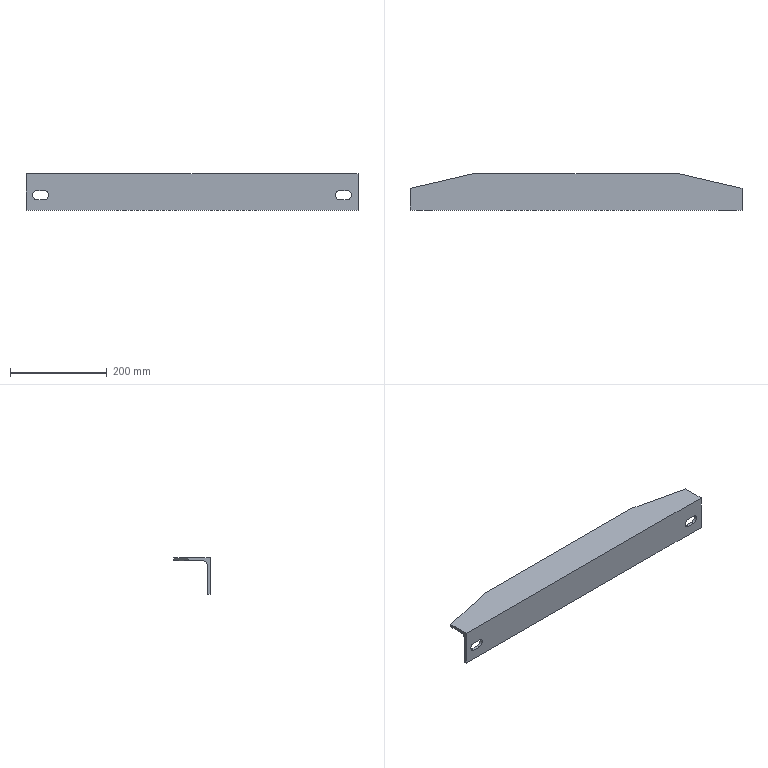Part | SolidWorks | features Chamfer 2, ICE 2, WeldMemberFeat 1, WeldmentFeature 1 | 1 solid | 21 faces | box 686 x 75 x 75 mm | volume 573977 mm3 | plane 14 | cylinder 7 | commonest cylinder face diameters 18 x5 4 x2
STEP:
#1=CARTESIAN_POINT('',(213.,75.,-4.));
#2=VERTEX_POINT('',#1);
#3=CARTESIAN_POINT('',(-213.,75.,-4.));
#4=VERTEX_POINT('',#3);
#5=CARTESIAN_POINT('',(343.,75.,-4.));
#6=DIRECTION('',(-1.,0.,0.));
#7=VECTOR('',#6,1000.);
#8=LINE('',#5,#7);
#9=EDGE_CURVE('',#2,#4,#8,.T.);
#10=ORIENTED_EDGE('',*,*,#9,.T.);
#11=CARTESIAN_POINT('',(-213.,75.,0.));
#12=VERTEX_POINT('',#11);
#13=CARTESIAN_POINT('',(-213.,75.,0.));
#14=DIRECTION('',(0.,0.,1.));
#15=VECTOR('',#14,1000.);
#16=LINE('',#13,#15);
#17=EDGE_CURVE('',#4,#12,#16,.T.);
#18=ORIENTED_EDGE('',*,*,#17,.T.);
#19=CARTESIAN_POINT('',(213.,75.,0.));
#20=VERTEX_POINT('',#19);
#21=CARTESIAN_POINT('',(343.,75.,0.));
#22=DIRECTION('',(-1.,0.,0.));
#23=VECTOR('',#22,1000.);
#24=LINE('',#21,#23);
#25=EDGE_CURVE('',#20,#12,#24,.T.);
#26=ORIENTED_EDGE('',*,*,#25,.F.);
#27=CARTESIAN_POINT('',(213.,75.,0.));
#28=DIRECTION('',(0.,0.,-1.));
#29=VECTOR('',#28,1000.);
#30=LINE('',#27,#29);
#31=EDGE_CURVE('',#20,#2,#30,.T.);
#32=ORIENTED_EDGE('',*,*,#31,.T.);
#33=EDGE_LOOP('',(#10,#18,#26,#32));
#34=FACE_OUTER_BOUND('',#33,.T.);
#35=CARTESIAN_POINT('',(343.,75.,0.));
#36=DIRECTION('',(0.,-1.,0.));
#37=DIRECTION('',(0.,0.,-1.));
#38=AXIS2_PLACEMENT_3D('',#35,#36,#37);
#39=PLANE('',#38);
#40=ADVANCED_FACE('',(#34),#39,.F.);
#41=ORIENTED_EDGE('',*,*,#25,.T.);
#42=CARTESIAN_POINT('',(-343.,45.,0.));
#43=VERTEX_POINT('',#42);
#44=CARTESIAN_POINT('',(-213.,75.,0.));
#45=DIRECTION('',(-0.9744,-0.2249,0.));
#46=VECTOR('',#45,1000.);
#47=LINE('',#44,#46);
#48=EDGE_CURVE('',#12,#43,#47,.T.);
#49=ORIENTED_EDGE('',*,*,#48,.T.);
#50=CARTESIAN_POINT('',(-343.,0.,0.));
#51=VERTEX_POINT('',#50);
#52=CARTESIAN_POINT('',(-343.,75.,0.));
#53=DIRECTION('',(0.,-1.,0.));
#54=VECTOR('',#53,1000.);
#55=LINE('',#52,#54);
#56=EDGE_CURVE('',#43,#51,#55,.T.);
#57=ORIENTED_EDGE('',*,*,#56,.T.);
#58=CARTESIAN_POINT('',(343.,0.,0.));
#59=VERTEX_POINT('',#58);
#60=CARTESIAN_POINT('',(343.,0.,0.));
#61=DIRECTION('',(-1.,0.,0.));
#62=VECTOR('',#61,1000.);
#63=LINE('',#60,#62);
#64=EDGE_CURVE('',#59,#51,#63,.T.);
#65=ORIENTED_EDGE('',*,*,#64,.F.);
#66=CARTESIAN_POINT('',(343.,45.,0.));
#67=VERTEX_POINT('',#66);
#68=CARTESIAN_POINT('',(343.,75.,0.));
#69=DIRECTION('',(0.,-1.,0.));
#70=VECTOR('',#69,1000.);
#71=LINE('',#68,#70);
#72=EDGE_CURVE('',#67,#59,#71,.T.);
#73=ORIENTED_EDGE('',*,*,#72,.F.);
#74=CARTESIAN_POINT('',(343.,45.,0.));
#75=DIRECTION('',(-0.9744,0.2249,0.));
#76=VECTOR('',#75,1000.);
#77=LINE('',#74,#76);
#78=EDGE_CURVE('',#67,#20,#77,.T.);
#79=ORIENTED_EDGE('',*,*,#78,.T.);
#80=EDGE_LOOP('',(#41,#49,#57,#65,#73,#79));
#81=FACE_OUTER_BOUND('',#80,.T.);
#82=CARTESIAN_POINT('',(343.,75.,0.));
#83=DIRECTION('',(0.,0.,-1.));
#84=DIRECTION('',(0.,1.,0.));
#85=AXIS2_PLACEMENT_3D('',#82,#83,#84);
#86=PLANE('',#85);
#87=ADVANCED_FACE('',(#81),#86,.F.);
#88=CARTESIAN_POINT('',(-320.5,0.,-53.));
#89=VERTEX_POINT('',#88);
#90=CARTESIAN_POINT('',(-305.5,0.,-53.));
#91=VERTEX_POINT('',#90);
#92=CARTESIAN_POINT('',(-320.5,0.,-53.));
#93=DIRECTION('',(1.,0.,0.));
#94=VECTOR('',#93,1000.);
#95=LINE('',#92,#94);
#96=EDGE_CURVE('',#89,#91,#95,.T.);
#97=ORIENTED_EDGE('',*,*,#96,.F.);
#98=CARTESIAN_POINT('',(-320.5,0.,-35.));
#99=VERTEX_POINT('',#98);
#100=CARTESIAN_POINT('',(-320.5,0.,-44.));
#101=DIRECTION('',(0.,-1.,0.));
#102=DIRECTION('',(0.,0.,1.));
#103=AXIS2_PLACEMENT_3D('',#100,#101,#102);
#104=CIRCLE('',#103,9.);
#105=EDGE_CURVE('',#99,#89,#104,.T.);
#106=ORIENTED_EDGE('',*,*,#105,.F.);
#107=CARTESIAN_POINT('',(-305.5,0.,-35.));
#108=VERTEX_POINT('',#107);
#109=CARTESIAN_POINT('',(-320.5,0.,-35.));
#110=DIRECTION('',(-1.,0.,0.));
#111=VECTOR('',#110,1000.);
#112=LINE('',#109,#111);
#113=EDGE_CURVE('',#108,#99,#112,.T.);
#114=ORIENTED_EDGE('',*,*,#113,.F.);
#115=CARTESIAN_POINT('',(-305.5,0.,-44.));
#116=DIRECTION('',(0.,-1.,0.));
#117=DIRECTION('',(0.,0.,1.));
#118=AXIS2_PLACEMENT_3D('',#115,#116,#117);
#119=CIRCLE('',#118,9.);
#120=EDGE_CURVE('',#91,#108,#119,.T.);
#121=ORIENTED_EDGE('',*,*,#120,.F.);
#122=EDGE_LOOP('',(#97,#106,#114,#121));
#123=FACE_BOUND('',#122,.T.);
#124=CARTESIAN_POINT('',(305.5,0.,-53.));
#125=VERTEX_POINT('',#124);
#126=CARTESIAN_POINT('',(320.5,0.,-53.));
#127=VERTEX_POINT('',#126);
#128=CARTESIAN_POINT('',(305.5,0.,-53.));
#129=DIRECTION('',(1.,0.,0.));
#130=VECTOR('',#129,1000.);
#131=LINE('',#128,#130);
#132=EDGE_CURVE('',#125,#127,#131,.T.);
#133=ORIENTED_EDGE('',*,*,#132,.F.);
#134=CARTESIAN_POINT('',(305.5,0.,-35.));
#135=VERTEX_POINT('',#134);
#136=CARTESIAN_POINT('',(305.5,0.,-44.));
#137=DIRECTION('',(0.,-1.,0.));
#138=DIRECTION('',(0.,0.,1.));
#139=AXIS2_PLACEMENT_3D('',#136,#137,#138);
#140=CIRCLE('',#139,9.);
#141=EDGE_CURVE('',#135,#125,#140,.T.);
#142=ORIENTED_EDGE('',*,*,#141,.F.);
#143=CARTESIAN_POINT('',(320.5,0.,-35.));
#144=VERTEX_POINT('',#143);
#145=CARTESIAN_POINT('',(305.5,0.,-35.));
#146=DIRECTION('',(-1.,0.,0.));
#147=VECTOR('',#146,1000.);
#148=LINE('',#145,#147);
#149=EDGE_CURVE('',#144,#135,#148,.T.);
#150=ORIENTED_EDGE('',*,*,#149,.F.);
#151=CARTESIAN_POINT('',(320.5,0.,-44.));
#152=DIRECTION('',(0.,-1.,0.));
#153=DIRECTION('',(0.,0.,1.));
#154=AXIS2_PLACEMENT_3D('',#151,#152,#153);
#155=CIRCLE('',#154,9.);
#156=EDGE_CURVE('',#127,#144,#155,.T.);
#157=ORIENTED_EDGE('',*,*,#156,.F.);
#158=EDGE_LOOP('',(#133,#142,#150,#157));
#159=FACE_BOUND('',#158,.T.);
#160=CARTESIAN_POINT('',(-343.,0.,-75.));
#161=VERTEX_POINT('',#160);
#162=CARTESIAN_POINT('',(-343.,0.,0.));
#163=DIRECTION('',(0.,0.,-1.));
#164=VECTOR('',#163,1000.);
#165=LINE('',#162,#164);
#166=EDGE_CURVE('',#51,#161,#165,.T.);
#167=ORIENTED_EDGE('',*,*,#166,.T.);
#168=CARTESIAN_POINT('',(343.,0.,-75.));
#169=VERTEX_POINT('',#168);
#170=CARTESIAN_POINT('',(343.,0.,-75.));
#171=DIRECTION('',(-1.,0.,0.));
#172=VECTOR('',#171,1000.);
#173=LINE('',#170,#172);
#174=EDGE_CURVE('',#169,#161,#173,.T.);
#175=ORIENTED_EDGE('',*,*,#174,.F.);
#176=CARTESIAN_POINT('',(343.,0.,0.));
#177=DIRECTION('',(0.,0.,-1.));
#178=VECTOR('',#177,1000.);
#179=LINE('',#176,#178);
#180=EDGE_CURVE('',#59,#169,#179,.T.);
#181=ORIENTED_EDGE('',*,*,#180,.F.);
#182=ORIENTED_EDGE('',*,*,#64,.T.);
#183=EDGE_LOOP('',(#167,#175,#181,#182));
#184=FACE_OUTER_BOUND('',#183,.T.);
#185=CARTESIAN_POINT('',(343.,0.,0.));
#186=DIRECTION('',(0.,1.,0.));
#187=DIRECTION('',(0.,0.,1.));
#188=AXIS2_PLACEMENT_3D('',#185,#186,#187);
#189=PLANE('',#188);
#190=ADVANCED_FACE('',(#123,#159,#184),#189,.F.);
#191=CARTESIAN_POINT('',(-343.,4.,-75.));
#192=VERTEX_POINT('',#191);
#193=CARTESIAN_POINT('',(-343.,0.,-75.));
#194=DIRECTION('',(0.,1.,0.));
#195=VECTOR('',#194,1000.);
#196=LINE('',#193,#195);
#197=EDGE_CURVE('',#161,#192,#196,.T.);
#198=ORIENTED_EDGE('',*,*,#197,.T.);
#199=CARTESIAN_POINT('',(343.,4.,-75.));
#200=VERTEX_POINT('',#199);
#201=CARTESIAN_POINT('',(343.,4.,-75.));
#202=DIRECTION('',(-1.,0.,0.));
#203=VECTOR('',#202,1000.);
#204=LINE('',#201,#203);
#205=EDGE_CURVE('',#200,#192,#204,.T.);
#206=ORIENTED_EDGE('',*,*,#205,.F.);
#207=CARTESIAN_POINT('',(343.,0.,-75.));
#208=DIRECTION('',(0.,1.,0.));
#209=VECTOR('',#208,1000.);
#210=LINE('',#207,#209);
#211=EDGE_CURVE('',#169,#200,#210,.T.);
#212=ORIENTED_EDGE('',*,*,#211,.F.);
#213=ORIENTED_EDGE('',*,*,#174,.T.);
#214=EDGE_LOOP('',(#198,#206,#212,#213));
#215=FACE_OUTER_BOUND('',#214,.T.);
#216=CARTESIAN_POINT('',(343.,0.,-75.));
#217=DIRECTION('',(0.,0.,1.));
#218=DIRECTION('',(0.,-1.,0.));
#219=AXIS2_PLACEMENT_3D('',#216,#217,#218);
#220=PLANE('',#219);
#221=ADVANCED_FACE('',(#215),#220,.F.);
#222=CARTESIAN_POINT('',(-343.,6.,-73.));
#223=VERTEX_POINT('',#222);
#224=CARTESIAN_POINT('',(-343.,4.,-73.));
#225=DIRECTION('',(1.,0.,0.));
#226=DIRECTION('',(0.,0.,-1.));
#227=AXIS2_PLACEMENT_3D('',#224,#225,#226);
#228=CIRCLE('',#227,2.);
#229=EDGE_CURVE('',#192,#223,#228,.T.);
#230=ORIENTED_EDGE('',*,*,#229,.T.);
#231=CARTESIAN_POINT('',(343.,6.,-73.));
#232=VERTEX_POINT('',#231);
#233=CARTESIAN_POINT('',(343.,6.,-73.));
#234=DIRECTION('',(-1.,0.,0.));
#235=VECTOR('',#234,1000.);
#236=LINE('',#233,#235);
#237=EDGE_CURVE('',#232,#223,#236,.T.);
#238=ORIENTED_EDGE('',*,*,#237,.F.);
#239=CARTESIAN_POINT('',(343.,4.,-73.));
#240=DIRECTION('',(1.,0.,0.));
#241=DIRECTION('',(0.,0.,-1.));
#242=AXIS2_PLACEMENT_3D('',#239,#240,#241);
#243=CIRCLE('',#242,2.);
#244=EDGE_CURVE('',#200,#232,#243,.T.);
#245=ORIENTED_EDGE('',*,*,#244,.F.);
#246=ORIENTED_EDGE('',*,*,#205,.T.);
#247=EDGE_LOOP('',(#230,#238,#245,#246));
#248=FACE_OUTER_BOUND('',#247,.T.);
#249=CARTESIAN_POINT('',(343.,4.,-73.));
#250=DIRECTION('',(-1.,0.,0.));
#251=DIRECTION('',(0.,0.,1.));
#252=AXIS2_PLACEMENT_3D('',#249,#250,#251);
#253=CYLINDRICAL_SURFACE('',#252,2.);
#254=ADVANCED_FACE('',(#248),#253,.T.);
#255=CARTESIAN_POINT('',(-320.5,6.,-35.));
#256=VERTEX_POINT('',#255);
#257=CARTESIAN_POINT('',(-305.5,6.,-35.));
#258=VERTEX_POINT('',#257);
#259=CARTESIAN_POINT('',(-320.5,6.,-35.));
#260=DIRECTION('',(1.,0.,0.));
#261=VECTOR('',#260,1000.);
#262=LINE('',#259,#261);
#263=EDGE_CURVE('',#256,#258,#262,.T.);
#264=ORIENTED_EDGE('',*,*,#263,.F.);
#265=CARTESIAN_POINT('',(-320.5,6.,-53.));
#266=VERTEX_POINT('',#265);
#267=CARTESIAN_POINT('',(-320.5,6.,-44.));
#268=DIRECTION('',(0.,1.,0.));
#269=DIRECTION('',(0.,0.,1.));
#270=AXIS2_PLACEMENT_3D('',#267,#268,#269);
#271=CIRCLE('',#270,9.);
#272=EDGE_CURVE('',#266,#256,#271,.T.);
#273=ORIENTED_EDGE('',*,*,#272,.F.);
#274=CARTESIAN_POINT('',(-305.5,6.,-53.));
#275=VERTEX_POINT('',#274);
#276=CARTESIAN_POINT('',(-320.5,6.,-53.));
#277=DIRECTION('',(-1.,0.,0.));
#278=VECTOR('',#277,1000.);
#279=LINE('',#276,#278);
#280=EDGE_CURVE('',#275,#266,#279,.T.);
#281=ORIENTED_EDGE('',*,*,#280,.F.);
#282=CARTESIAN_POINT('',(-305.5,6.,-44.));
#283=DIRECTION('',(0.,1.,0.));
#284=DIRECTION('',(0.,0.,1.));
#285=AXIS2_PLACEMENT_3D('',#282,#283,#284);
#286=CIRCLE('',#285,9.);
#287=EDGE_CURVE('',#258,#275,#286,.T.);
#288=ORIENTED_EDGE('',*,*,#287,.F.);
#289=EDGE_LOOP('',(#264,#273,#281,#288));
#290=FACE_BOUND('',#289,.T.);
#291=CARTESIAN_POINT('',(305.5,6.,-35.));
#292=VERTEX_POINT('',#291);
#293=CARTESIAN_POINT('',(320.5,6.,-35.));
#294=VERTEX_POINT('',#293);
#295=CARTESIAN_POINT('',(305.5,6.,-35.));
#296=DIRECTION('',(1.,0.,0.));
#297=VECTOR('',#296,1000.);
#298=LINE('',#295,#297);
#299=EDGE_CURVE('',#292,#294,#298,.T.);
#300=ORIENTED_EDGE('',*,*,#299,.F.);
#301=CARTESIAN_POINT('',(305.5,6.,-53.));
#302=VERTEX_POINT('',#301);
#303=CARTESIAN_POINT('',(305.5,6.,-44.));
#304=DIRECTION('',(0.,1.,0.));
#305=DIRECTION('',(0.,0.,1.));
#306=AXIS2_PLACEMENT_3D('',#303,#304,#305);
#307=CIRCLE('',#306,9.);
#308=EDGE_CURVE('',#302,#292,#307,.T.);
#309=ORIENTED_EDGE('',*,*,#308,.F.);
#310=CARTESIAN_POINT('',(320.5,6.,-53.));
#311=VERTEX_POINT('',#310);
#312=CARTESIAN_POINT('',(305.5,6.,-53.));
#313=DIRECTION('',(-1.,0.,0.));
#314=VECTOR('',#313,1000.);
#315=LINE('',#312,#314);
#316=EDGE_CURVE('',#311,#302,#315,.T.);
#317=ORIENTED_EDGE('',*,*,#316,.F.);
#318=CARTESIAN_POINT('',(320.5,6.,-44.));
#319=DIRECTION('',(0.,1.,0.));
#320=DIRECTION('',(0.,0.,1.));
#321=AXIS2_PLACEMENT_3D('',#318,#319,#320);
#322=CIRCLE('',#321,9.);
#323=EDGE_CURVE('',#294,#311,#322,.T.);
#324=ORIENTED_EDGE('',*,*,#323,.F.);
#325=EDGE_LOOP('',(#300,#309,#317,#324));
#326=FACE_BOUND('',#325,.T.);
#327=CARTESIAN_POINT('',(-343.,6.,-15.));
#328=VERTEX_POINT('',#327);
#329=CARTESIAN_POINT('',(-343.,6.,-15.));
#330=DIRECTION('',(0.,0.,1.));
#331=VECTOR('',#330,1000.);
#332=LINE('',#329,#331);
#333=EDGE_CURVE('',#223,#328,#332,.T.);
#334=ORIENTED_EDGE('',*,*,#333,.T.);
#335=CARTESIAN_POINT('',(343.,6.,-15.));
#336=VERTEX_POINT('',#335);
#337=CARTESIAN_POINT('',(343.,6.,-15.));
#338=DIRECTION('',(-1.,0.,0.));
#339=VECTOR('',#338,1000.);
#340=LINE('',#337,#339);
#341=EDGE_CURVE('',#336,#328,#340,.T.);
#342=ORIENTED_EDGE('',*,*,#341,.F.);
#343=CARTESIAN_POINT('',(343.,6.,-15.));
#344=DIRECTION('',(0.,0.,1.));
#345=VECTOR('',#344,1000.);
#346=LINE('',#343,#345);
#347=EDGE_CURVE('',#232,#336,#346,.T.);
#348=ORIENTED_EDGE('',*,*,#347,.F.);
#349=ORIENTED_EDGE('',*,*,#237,.T.);
#350=EDGE_LOOP('',(#334,#342,#348,#349));
#351=FACE_OUTER_BOUND('',#350,.T.);
#352=CARTESIAN_POINT('',(343.,6.,-15.));
#353=DIRECTION('',(0.,-1.,0.));
#354=DIRECTION('',(0.,0.,-1.));
#355=AXIS2_PLACEMENT_3D('',#352,#353,#354);
#356=PLANE('',#355);
#357=ADVANCED_FACE('',(#290,#326,#351),#356,.F.);
#358=CARTESIAN_POINT('',(-343.,15.,-6.));
#359=VERTEX_POINT('',#358);
#360=CARTESIAN_POINT('',(-343.,15.,-15.));
#361=DIRECTION('',(-1.,0.,0.));
#362=DIRECTION('',(0.,0.,-1.));
#363=AXIS2_PLACEMENT_3D('',#360,#361,#362);
#364=CIRCLE('',#363,9.);
#365=EDGE_CURVE('',#328,#359,#364,.T.);
#366=ORIENTED_EDGE('',*,*,#365,.T.);
#367=CARTESIAN_POINT('',(343.,15.,-6.));
#368=VERTEX_POINT('',#367);
#369=CARTESIAN_POINT('',(343.,15.,-6.));
#370=DIRECTION('',(-1.,0.,0.));
#371=VECTOR('',#370,1000.);
#372=LINE('',#369,#371);
#373=EDGE_CURVE('',#368,#359,#372,.T.);
#374=ORIENTED_EDGE('',*,*,#373,.F.);
#375=CARTESIAN_POINT('',(343.,15.,-15.));
#376=DIRECTION('',(-1.,0.,0.));
#377=DIRECTION('',(0.,0.,-1.));
#378=AXIS2_PLACEMENT_3D('',#375,#376,#377);
#379=CIRCLE('',#378,9.);
#380=EDGE_CURVE('',#336,#368,#379,.T.);
#381=ORIENTED_EDGE('',*,*,#380,.F.);
#382=ORIENTED_EDGE('',*,*,#341,.T.);
#383=EDGE_LOOP('',(#366,#374,#381,#382));
#384=FACE_OUTER_BOUND('',#383,.T.);
#385=CARTESIAN_POINT('',(343.,15.,-15.));
#386=DIRECTION('',(-1.,0.,0.));
#387=DIRECTION('',(0.,0.,1.));
#388=AXIS2_PLACEMENT_3D('',#385,#386,#387);
#389=CYLINDRICAL_SURFACE('',#388,9.);
#390=ADVANCED_FACE('',(#384),#389,.F.);
#391=CARTESIAN_POINT('',(-343.,45.,-6.));
#392=VERTEX_POINT('',#391);
#393=CARTESIAN_POINT('',(-343.,73.,-6.));
#394=DIRECTION('',(0.,1.,0.));
#395=VECTOR('',#394,1000.);
#396=LINE('',#393,#395);
#397=EDGE_CURVE('',#359,#392,#396,.T.);
#398=ORIENTED_EDGE('',*,*,#397,.T.);
#399=CARTESIAN_POINT('',(-221.667,73.,-6.));
#400=VERTEX_POINT('',#399);
#401=CARTESIAN_POINT('',(-213.,75.,-6.));
#402=DIRECTION('',(0.9744,0.2249,0.));
#403=VECTOR('',#402,1000.);
#404=LINE('',#401,#403);
#405=EDGE_CURVE('',#392,#400,#404,.T.);
#406=ORIENTED_EDGE('',*,*,#405,.T.);
#407=CARTESIAN_POINT('',(221.667,73.,-6.));
#408=VERTEX_POINT('',#407);
#409=CARTESIAN_POINT('',(343.,73.,-6.));
#410=DIRECTION('',(-1.,0.,0.));
#411=VECTOR('',#410,1000.);
#412=LINE('',#409,#411);
#413=EDGE_CURVE('',#408,#400,#412,.T.);
#414=ORIENTED_EDGE('',*,*,#413,.F.);
#415=CARTESIAN_POINT('',(343.,45.,-6.));
#416=VERTEX_POINT('',#415);
#417=CARTESIAN_POINT('',(343.,45.,-6.));
#418=DIRECTION('',(0.9744,-0.2249,0.));
#419=VECTOR('',#418,1000.);
#420=LINE('',#417,#419);
#421=EDGE_CURVE('',#408,#416,#420,.T.);
#422=ORIENTED_EDGE('',*,*,#421,.T.);
#423=CARTESIAN_POINT('',(343.,73.,-6.));
#424=DIRECTION('',(0.,1.,0.));
#425=VECTOR('',#424,1000.);
#426=LINE('',#423,#425);
#427=EDGE_CURVE('',#368,#416,#426,.T.);
#428=ORIENTED_EDGE('',*,*,#427,.F.);
#429=ORIENTED_EDGE('',*,*,#373,.T.);
#430=EDGE_LOOP('',(#398,#406,#414,#422,#428,#429));
#431=FACE_OUTER_BOUND('',#430,.T.);
#432=CARTESIAN_POINT('',(343.,73.,-6.));
#433=DIRECTION('',(0.,0.,1.));
#434=DIRECTION('',(0.,-1.,0.));
#435=AXIS2_PLACEMENT_3D('',#432,#433,#434);
#436=PLANE('',#435);
#437=ADVANCED_FACE('',(#431),#436,.F.);
#438=ORIENTED_EDGE('',*,*,#413,.T.);
#439=CARTESIAN_POINT('',(-221.667,73.,-6.));
#440=CARTESIAN_POINT('',(-216.59,74.172,-6.));
#441=CARTESIAN_POINT('',(-213.,75.,-5.172));
#442=CARTESIAN_POINT('',(-213.,75.,-4.));
#443=(BOUNDED_CURVE()B_SPLINE_CURVE(3,(#439,#440,#441,#442),.UNSPECIFIED.,.F.,.T.)B_SPLINE_CURVE_WITH_KNOTS((4,4),(1.571,3.142),.UNSPECIFIED.)CURVE()GEOMETRIC_REPRESENTATION_ITEM()RATIONAL_B_SPLINE_CURVE((1.,0.8047,0.8047,1.))REPRESENTATION_ITEM(''));
#444=EDGE_CURVE('',#400,#4,#443,.T.);
#445=ORIENTED_EDGE('',*,*,#444,.T.);
#446=ORIENTED_EDGE('',*,*,#9,.F.);
#447=CARTESIAN_POINT('',(213.,75.,-4.));
#448=CARTESIAN_POINT('',(213.,75.,-5.172));
#449=CARTESIAN_POINT('',(216.59,74.172,-6.));
#450=CARTESIAN_POINT('',(221.667,73.,-6.));
#451=(BOUNDED_CURVE()B_SPLINE_CURVE(3,(#447,#448,#449,#450),.UNSPECIFIED.,.F.,.T.)B_SPLINE_CURVE_WITH_KNOTS((4,4),(0.,1.571),.UNSPECIFIED.)CURVE()GEOMETRIC_REPRESENTATION_ITEM()RATIONAL_B_SPLINE_CURVE((1.,0.8047,0.8047,1.))REPRESENTATION_ITEM(''));
#452=EDGE_CURVE('',#2,#408,#451,.T.);
#453=ORIENTED_EDGE('',*,*,#452,.T.);
#454=EDGE_LOOP('',(#438,#445,#446,#453));
#455=FACE_OUTER_BOUND('',#454,.T.);
#456=CARTESIAN_POINT('',(343.,73.,-4.));
#457=DIRECTION('',(-1.,0.,0.));
#458=DIRECTION('',(0.,0.,1.));
#459=AXIS2_PLACEMENT_3D('',#456,#457,#458);
#460=CYLINDRICAL_SURFACE('',#459,2.);
#461=ADVANCED_FACE('',(#455),#460,.T.);
#462=ORIENTED_EDGE('',*,*,#427,.T.);
#463=CARTESIAN_POINT('',(343.,45.,-4.));
#464=DIRECTION('',(0.,0.,1.));
#465=VECTOR('',#464,1000.);
#466=LINE('',#463,#465);
#467=EDGE_CURVE('',#416,#67,#466,.T.);
#468=ORIENTED_EDGE('',*,*,#467,.T.);
#469=ORIENTED_EDGE('',*,*,#72,.T.);
#470=ORIENTED_EDGE('',*,*,#180,.T.);
#471=ORIENTED_EDGE('',*,*,#211,.T.);
#472=ORIENTED_EDGE('',*,*,#244,.T.);
#473=ORIENTED_EDGE('',*,*,#347,.T.);
#474=ORIENTED_EDGE('',*,*,#380,.T.);
#475=EDGE_LOOP('',(#462,#468,#469,#470,#471,#472,#473,#474));
#476=FACE_OUTER_BOUND('',#475,.T.);
#477=CARTESIAN_POINT('',(343.,73.,-4.));
#478=DIRECTION('',(-1.,0.,0.));
#479=DIRECTION('',(0.,0.,1.));
#480=AXIS2_PLACEMENT_3D('',#477,#478,#479);
#481=PLANE('',#480);
#482=ADVANCED_FACE('',(#476),#481,.F.);
#483=ORIENTED_EDGE('',*,*,#56,.F.);
#484=CARTESIAN_POINT('',(-343.,45.,-4.));
#485=DIRECTION('',(0.,0.,-1.));
#486=VECTOR('',#485,1000.);
#487=LINE('',#484,#486);
#488=EDGE_CURVE('',#43,#392,#487,.T.);
#489=ORIENTED_EDGE('',*,*,#488,.T.);
#490=ORIENTED_EDGE('',*,*,#397,.F.);
#491=ORIENTED_EDGE('',*,*,#365,.F.);
#492=ORIENTED_EDGE('',*,*,#333,.F.);
#493=ORIENTED_EDGE('',*,*,#229,.F.);
#494=ORIENTED_EDGE('',*,*,#197,.F.);
#495=ORIENTED_EDGE('',*,*,#166,.F.);
#496=EDGE_LOOP('',(#483,#489,#490,#491,#492,#493,#494,#495));
#497=FACE_OUTER_BOUND('',#496,.T.);
#498=CARTESIAN_POINT('',(-343.,73.,-4.));
#499=DIRECTION('',(-1.,0.,0.));
#500=DIRECTION('',(0.,0.,1.));
#501=AXIS2_PLACEMENT_3D('',#498,#499,#500);
#502=PLANE('',#501);
#503=ADVANCED_FACE('',(#497),#502,.T.);
#504=ORIENTED_EDGE('',*,*,#141,.T.);
#505=CARTESIAN_POINT('',(305.5,-0.001,-53.));
#506=DIRECTION('',(0.,1.,0.));
#507=VECTOR('',#506,1000.);
#508=LINE('',#505,#507);
#509=EDGE_CURVE('',#125,#302,#508,.T.);
#510=ORIENTED_EDGE('',*,*,#509,.T.);
#511=ORIENTED_EDGE('',*,*,#308,.T.);
#512=CARTESIAN_POINT('',(305.5,-0.001,-35.));
#513=DIRECTION('',(0.,1.,0.));
#514=VECTOR('',#513,1000.);
#515=LINE('',#512,#514);
#516=EDGE_CURVE('',#135,#292,#515,.T.);
#517=ORIENTED_EDGE('',*,*,#516,.F.);
#518=EDGE_LOOP('',(#504,#510,#511,#517));
#519=FACE_OUTER_BOUND('',#518,.T.);
#520=CARTESIAN_POINT('',(305.5,-0.001,-44.));
#521=DIRECTION('',(0.,1.,0.));
#522=DIRECTION('',(0.,0.,1.));
#523=AXIS2_PLACEMENT_3D('',#520,#521,#522);
#524=CYLINDRICAL_SURFACE('',#523,9.);
#525=ADVANCED_FACE('',(#519),#524,.F.);
#526=ORIENTED_EDGE('',*,*,#132,.T.);
#527=CARTESIAN_POINT('',(320.5,-0.001,-53.));
#528=DIRECTION('',(0.,1.,0.));
#529=VECTOR('',#528,1000.);
#530=LINE('',#527,#529);
#531=EDGE_CURVE('',#127,#311,#530,.T.);
#532=ORIENTED_EDGE('',*,*,#531,.T.);
#533=ORIENTED_EDGE('',*,*,#316,.T.);
#534=ORIENTED_EDGE('',*,*,#509,.F.);
#535=EDGE_LOOP('',(#526,#532,#533,#534));
#536=FACE_OUTER_BOUND('',#535,.T.);
#537=CARTESIAN_POINT('',(305.5,-0.001,-53.));
#538=DIRECTION('',(0.,0.,-1.));
#539=DIRECTION('',(0.,1.,0.));
#540=AXIS2_PLACEMENT_3D('',#537,#538,#539);
#541=PLANE('',#540);
#542=ADVANCED_FACE('',(#536),#541,.F.);
#543=ORIENTED_EDGE('',*,*,#156,.T.);
#544=CARTESIAN_POINT('',(320.5,-0.001,-35.));
#545=DIRECTION('',(0.,1.,0.));
#546=VECTOR('',#545,1000.);
#547=LINE('',#544,#546);
#548=EDGE_CURVE('',#144,#294,#547,.T.);
#549=ORIENTED_EDGE('',*,*,#548,.T.);
#550=ORIENTED_EDGE('',*,*,#323,.T.);
#551=ORIENTED_EDGE('',*,*,#531,.F.);
#552=EDGE_LOOP('',(#543,#549,#550,#551));
#553=FACE_OUTER_BOUND('',#552,.T.);
#554=CARTESIAN_POINT('',(320.5,-0.001,-44.));
#555=DIRECTION('',(0.,1.,0.));
#556=DIRECTION('',(0.,0.,1.));
#557=AXIS2_PLACEMENT_3D('',#554,#555,#556);
#558=CYLINDRICAL_SURFACE('',#557,9.);
#559=ADVANCED_FACE('',(#553),#558,.F.);
#560=ORIENTED_EDGE('',*,*,#149,.T.);
#561=ORIENTED_EDGE('',*,*,#516,.T.);
#562=ORIENTED_EDGE('',*,*,#299,.T.);
#563=ORIENTED_EDGE('',*,*,#548,.F.);
#564=EDGE_LOOP('',(#560,#561,#562,#563));
#565=FACE_OUTER_BOUND('',#564,.T.);
#566=CARTESIAN_POINT('',(305.5,-0.001,-35.));
#567=DIRECTION('',(0.,0.,1.));
#568=DIRECTION('',(1.,0.,0.));
#569=AXIS2_PLACEMENT_3D('',#566,#567,#568);
#570=PLANE('',#569);
#571=ADVANCED_FACE('',(#565),#570,.F.);
#572=ORIENTED_EDGE('',*,*,#105,.T.);
#573=CARTESIAN_POINT('',(-320.5,-0.001,-53.));
#574=DIRECTION('',(0.,1.,0.));
#575=VECTOR('',#574,1000.);
#576=LINE('',#573,#575);
#577=EDGE_CURVE('',#89,#266,#576,.T.);
#578=ORIENTED_EDGE('',*,*,#577,.T.);
#579=ORIENTED_EDGE('',*,*,#272,.T.);
#580=CARTESIAN_POINT('',(-320.5,-0.001,-35.));
#581=DIRECTION('',(0.,1.,0.));
#582=VECTOR('',#581,1000.);
#583=LINE('',#580,#582);
#584=EDGE_CURVE('',#99,#256,#583,.T.);
#585=ORIENTED_EDGE('',*,*,#584,.F.);
#586=EDGE_LOOP('',(#572,#578,#579,#585));
#587=FACE_OUTER_BOUND('',#586,.T.);
#588=CARTESIAN_POINT('',(-320.5,-0.001,-44.));
#589=DIRECTION('',(0.,1.,0.));
#590=DIRECTION('',(0.,0.,1.));
#591=AXIS2_PLACEMENT_3D('',#588,#589,#590);
#592=CYLINDRICAL_SURFACE('',#591,9.);
#593=ADVANCED_FACE('',(#587),#592,.F.);
#594=ORIENTED_EDGE('',*,*,#96,.T.);
#595=CARTESIAN_POINT('',(-305.5,-0.001,-53.));
#596=DIRECTION('',(0.,1.,0.));
#597=VECTOR('',#596,1000.);
#598=LINE('',#595,#597);
#599=EDGE_CURVE('',#91,#275,#598,.T.);
#600=ORIENTED_EDGE('',*,*,#599,.T.);
#601=ORIENTED_EDGE('',*,*,#280,.T.);
#602=ORIENTED_EDGE('',*,*,#577,.F.);
#603=EDGE_LOOP('',(#594,#600,#601,#602));
#604=FACE_OUTER_BOUND('',#603,.T.);
#605=CARTESIAN_POINT('',(-320.5,-0.001,-53.));
#606=DIRECTION('',(0.,0.,-1.));
#607=DIRECTION('',(-1.,0.,0.));
#608=AXIS2_PLACEMENT_3D('',#605,#606,#607);
#609=PLANE('',#608);
#610=ADVANCED_FACE('',(#604),#609,.F.);
#611=ORIENTED_EDGE('',*,*,#120,.T.);
#612=CARTESIAN_POINT('',(-305.5,-0.001,-35.));
#613=DIRECTION('',(0.,1.,0.));
#614=VECTOR('',#613,1000.);
#615=LINE('',#612,#614);
#616=EDGE_CURVE('',#108,#258,#615,.T.);
#617=ORIENTED_EDGE('',*,*,#616,.T.);
#618=ORIENTED_EDGE('',*,*,#287,.T.);
#619=ORIENTED_EDGE('',*,*,#599,.F.);
#620=EDGE_LOOP('',(#611,#617,#618,#619));
#621=FACE_OUTER_BOUND('',#620,.T.);
#622=CARTESIAN_POINT('',(-305.5,-0.001,-44.));
#623=DIRECTION('',(0.,1.,0.));
#624=DIRECTION('',(0.,0.,1.));
#625=AXIS2_PLACEMENT_3D('',#622,#623,#624);
#626=CYLINDRICAL_SURFACE('',#625,9.);
#627=ADVANCED_FACE('',(#621),#626,.F.);
#628=ORIENTED_EDGE('',*,*,#113,.T.);
#629=ORIENTED_EDGE('',*,*,#584,.T.);
#630=ORIENTED_EDGE('',*,*,#263,.T.);
#631=ORIENTED_EDGE('',*,*,#616,.F.);
#632=EDGE_LOOP('',(#628,#629,#630,#631));
#633=FACE_OUTER_BOUND('',#632,.T.);
#634=CARTESIAN_POINT('',(-320.5,-0.001,-35.));
#635=DIRECTION('',(0.,0.,1.));
#636=DIRECTION('',(0.,-1.,0.));
#637=AXIS2_PLACEMENT_3D('',#634,#635,#636);
#638=PLANE('',#637);
#639=ADVANCED_FACE('',(#633),#638,.F.);
#640=ORIENTED_EDGE('',*,*,#452,.F.);
#641=ORIENTED_EDGE('',*,*,#31,.F.);
#642=ORIENTED_EDGE('',*,*,#78,.F.);
#643=ORIENTED_EDGE('',*,*,#467,.F.);
#644=ORIENTED_EDGE('',*,*,#421,.F.);
#645=EDGE_LOOP('',(#640,#641,#642,#643,#644));
#646=FACE_OUTER_BOUND('',#645,.T.);
#647=CARTESIAN_POINT('',(343.,45.,-4.));
#648=DIRECTION('',(-0.2249,-0.9744,0.));
#649=DIRECTION('',(0.,0.,1.));
#650=AXIS2_PLACEMENT_3D('',#647,#648,#649);
#651=PLANE('',#650);
#652=ADVANCED_FACE('',(#646),#651,.F.);
#653=ORIENTED_EDGE('',*,*,#405,.F.);
#654=ORIENTED_EDGE('',*,*,#488,.F.);
#655=ORIENTED_EDGE('',*,*,#48,.F.);
#656=ORIENTED_EDGE('',*,*,#17,.F.);
#657=ORIENTED_EDGE('',*,*,#444,.F.);
#658=EDGE_LOOP('',(#653,#654,#655,#656,#657));
#659=FACE_OUTER_BOUND('',#658,.T.);
#660=CARTESIAN_POINT('',(-213.,75.,0.));
#661=DIRECTION('',(-0.2249,0.9744,0.));
#662=DIRECTION('',(0.,0.,-1.));
#663=AXIS2_PLACEMENT_3D('',#660,#661,#662);
#664=PLANE('',#663);
#665=ADVANCED_FACE('',(#659),#664,.T.);
#666=CLOSED_SHELL('',(#40,#87,#190,#221,#254,#357,#390,#437,#461,#482,#503,#525,#542,#559,#571,#593,#610,#627,#639,#652,#665));
#667=MANIFOLD_SOLID_BREP('',#666);
#668=CARTESIAN_POINT('',(0.,0.,0.));
#669=DIRECTION('',(0.,0.,1.));
#670=DIRECTION('',(1.,0.,0.));
#671=AXIS2_PLACEMENT_3D('',#668,#669,#670);
#672=(LENGTH_UNIT()NAMED_UNIT(*)SI_UNIT(.MILLI.,.METRE.));
#673=UNCERTAINTY_MEASURE_WITH_UNIT(LENGTH_MEASURE(0.00001),#672,'','');
#674=(NAMED_UNIT(*)PLANE_ANGLE_UNIT()SI_UNIT($,.RADIAN.));
#675=(NAMED_UNIT(*)SI_UNIT($,.STERADIAN.)SOLID_ANGLE_UNIT());
#676=(GEOMETRIC_REPRESENTATION_CONTEXT(3)GLOBAL_UNCERTAINTY_ASSIGNED_CONTEXT((#673))GLOBAL_UNIT_ASSIGNED_CONTEXT((#672,#674,#675))REPRESENTATION_CONTEXT('',''));
#677=ADVANCED_BREP_SHAPE_REPRESENTATION('',(#667,#671),#676);